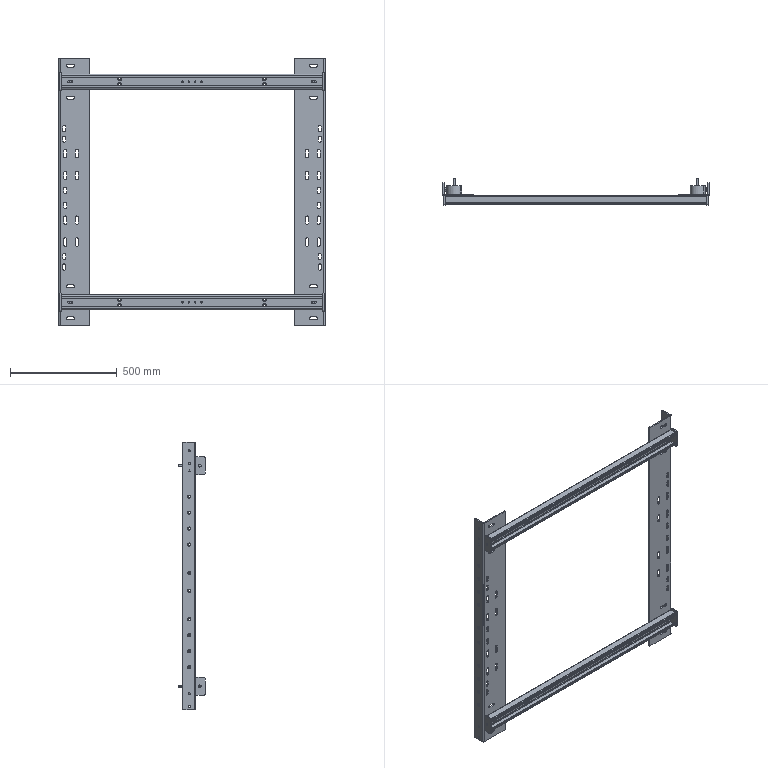Part | 40 solids | 1266 faces | box 1250 x 124 x 1255 mm | volume 4426852 mm3 | plane 666 | cylinder 432 | cone 168 | commonest cylinder face diameters 10.647 x56 14.75 x56 15.07 x56 13 x52 14 x48 15 x40